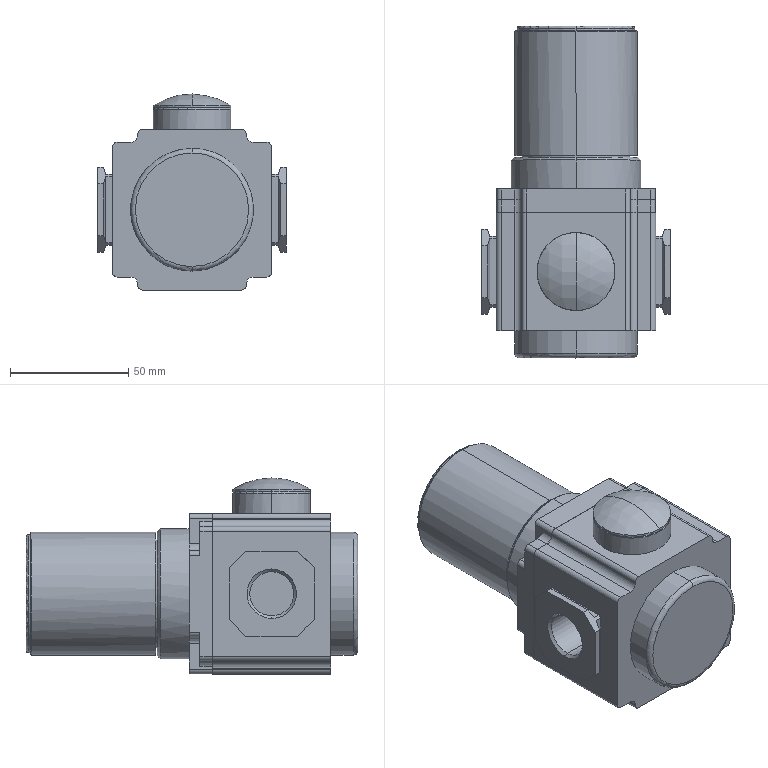Part | SolidWorks | features BaseBody 1 | 1 solid | 142 faces | box 80 x 140.5 x 83 mm | volume 444792 mm3 | plane 76 | cylinder 50 | cone 8 | torus 6 | sphere 2 | commonest cylinder face diameters 4 x20 6 x12 18.631 x4 33 x4 52 x4 45.9 x2